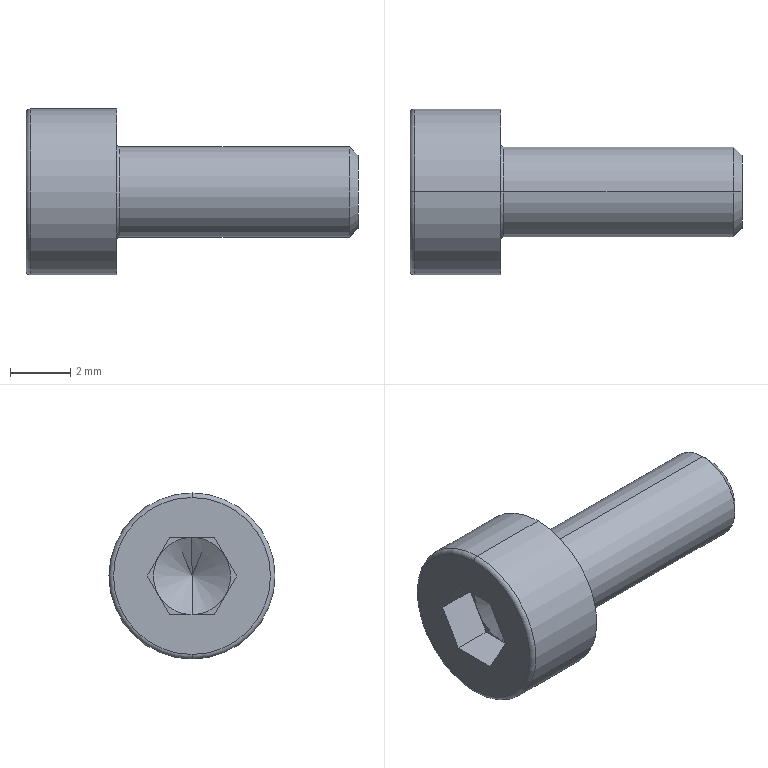Part | STEP file | socket head cap screw_iso_ISO 4762 M3 x 8 --- 8N | 1 solid | 27 faces | box 11 x 5.5 x 5.5 mm | volume 118.768 mm3 | plane 15 | cone 4 | torus 4 | cylinder 4 | commonest cylinder face diameters 3 x2 5.5 x2